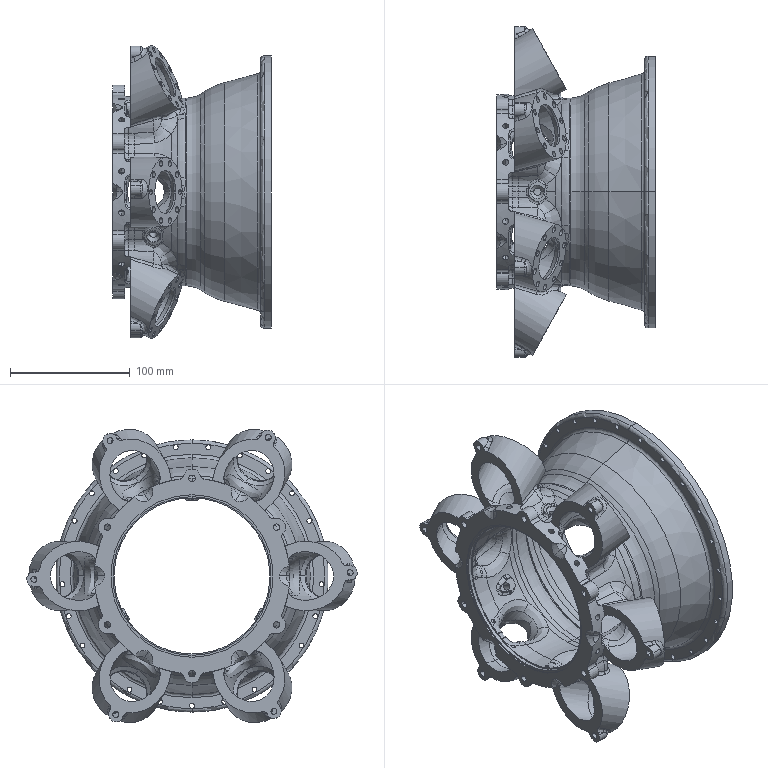Part | STEP file | Completa.sldasm-Part-24_Valor predeterminado | 1 solid | 1090 faces | box 132.616 x 276.232 x 245.091 mm | volume 834308 mm3 | cylinder 395 | spline 291 | plane 146 | torus 129 | cone 77 | sphere 48 | other 4 | commonest cylinder face diameters 5 x162 4.11 x50 6.4 x14 4 x12 5.4 x12 12 x12